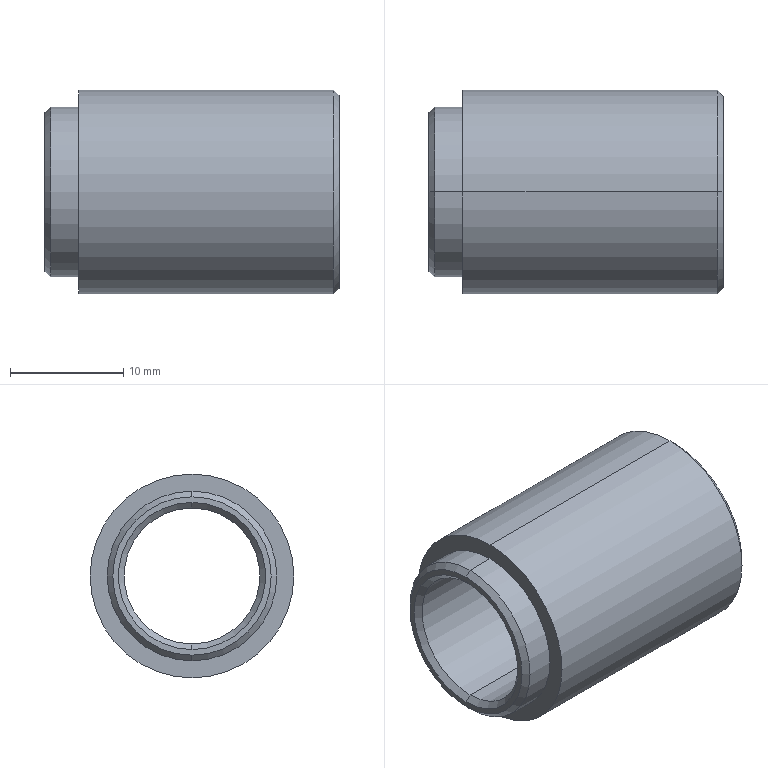Part | STEP file | 8XS210010 | 1 solid | 17 faces | box 26 x 18 x 18 mm | volume 3420 mm3 | cone 8 | cylinder 6 | plane 3 | commonest cylinder face diameters 12 x2 15 x2 18 x2
STEP:
#1=CARTESIAN_POINT('',(0.,0.,0.));
#2=DIRECTION('',(0.,0.,1.));
#3=DIRECTION('',(1.,0.,0.));
#4=AXIS2_PLACEMENT_3D('',#1,#2,#3);
#5=CARTESIAN_POINT('',(3.,0.,-9.));
#6=VERTEX_POINT('',#5);
#7=CARTESIAN_POINT('',(3.,0.,9.));
#8=VERTEX_POINT('',#7);
#9=CARTESIAN_POINT('',(3.,0.,0.));
#10=DIRECTION('',(1.,0.,0.));
#11=DIRECTION('',(0.,0.,-1.));
#12=AXIS2_PLACEMENT_3D('',#9,#10,#11);
#13=CIRCLE('',#12,9.);
#14=CARTESIAN_POINT('',(14.5,0.,0.));
#15=DIRECTION('',(1.,0.,0.));
#16=DIRECTION('',(0.,0.,-1.));
#17=AXIS2_PLACEMENT_3D('',#14,#15,#16);
#18=CYLINDRICAL_SURFACE('',#17,9.);
#19=CARTESIAN_POINT('',(0.,-11.5));
#20=DIRECTION('',(1.,0.));
#21=VECTOR('',#20,1.);
#22=LINE('',#19,#21);
#23=(GEOMETRIC_REPRESENTATION_CONTEXT(2)PARAMETRIC_REPRESENTATION_CONTEXT()REPRESENTATION_CONTEXT('',''));
#24=DEFINITIONAL_REPRESENTATION('',(#22),#23);
#25=PCURVE('',#18,#24);
#26=CARTESIAN_POINT('',(3.,8.25,0.));
#27=DIRECTION('',(-1.,0.,0.));
#28=DIRECTION('',(0.,0.,1.));
#29=AXIS2_PLACEMENT_3D('',#26,#27,#28);
#30=PLANE('',#29);
#31=CARTESIAN_POINT('',(-9.,-8.25));
#32=CARTESIAN_POINT('',(-9.,7.338));
#33=CARTESIAN_POINT('',(4.5,-0.4558));
#34=CARTESIAN_POINT('',(18.,-8.25));
#35=CARTESIAN_POINT('',(4.5,-16.044));
#36=CARTESIAN_POINT('',(-9.,-23.838));
#37=CARTESIAN_POINT('',(-9.,-8.25));
#38=(BOUNDED_CURVE()B_SPLINE_CURVE(2,(#31,#32,#33,#34,#35,#36,#37),.UNSPECIFIED.,.T.,.F.)B_SPLINE_CURVE_WITH_KNOTS((1,2,2,2,2,1),(-2.094,0.,2.094,4.189,6.283,8.378),.UNSPECIFIED.)CURVE()GEOMETRIC_REPRESENTATION_ITEM()RATIONAL_B_SPLINE_CURVE((1.,0.5,1.,0.5,1.,0.5,1.))REPRESENTATION_ITEM(''));
#39=(GEOMETRIC_REPRESENTATION_CONTEXT(2)PARAMETRIC_REPRESENTATION_CONTEXT()REPRESENTATION_CONTEXT('',''));
#40=DEFINITIONAL_REPRESENTATION('',(#38),#39);
#41=PCURVE('',#30,#40);
#42=SURFACE_CURVE('',#13,(#25,#41),.PCURVE_S1.);
#43=EDGE_CURVE('',#6,#8,#42,.T.);
#44=ORIENTED_EDGE('',*,*,#43,.T.);
#45=CARTESIAN_POINT('',(25.5,0.,9.));
#46=VERTEX_POINT('',#45);
#47=CARTESIAN_POINT('',(14.5,0.,9.));
#48=DIRECTION('',(1.,0.,0.));
#49=VECTOR('',#48,1.);
#50=LINE('',#47,#49);
#51=CARTESIAN_POINT('',(3.142,0.));
#52=DIRECTION('',(0.,1.));
#53=VECTOR('',#52,1.);
#54=LINE('',#51,#53);
#55=(GEOMETRIC_REPRESENTATION_CONTEXT(2)PARAMETRIC_REPRESENTATION_CONTEXT()REPRESENTATION_CONTEXT('',''));
#56=DEFINITIONAL_REPRESENTATION('',(#54),#55);
#57=PCURVE('',#18,#56);
#58=CARTESIAN_POINT('',(14.5,0.,0.));
#59=DIRECTION('',(1.,0.,0.));
#60=DIRECTION('',(0.,0.,-1.));
#61=AXIS2_PLACEMENT_3D('',#58,#59,#60);
#62=CYLINDRICAL_SURFACE('',#61,9.);
#63=CARTESIAN_POINT('',(3.142,0.));
#64=DIRECTION('',(0.,1.));
#65=VECTOR('',#64,1.);
#66=LINE('',#63,#65);
#67=(GEOMETRIC_REPRESENTATION_CONTEXT(2)PARAMETRIC_REPRESENTATION_CONTEXT()REPRESENTATION_CONTEXT('',''));
#68=DEFINITIONAL_REPRESENTATION('',(#66),#67);
#69=PCURVE('',#62,#68);
#70=SURFACE_CURVE('',#50,(#57,#69),.PCURVE_S1.);
#71=EDGE_CURVE('',#8,#46,#70,.T.);
#72=ORIENTED_EDGE('',*,*,#71,.T.);
#73=CARTESIAN_POINT('',(25.5,0.,-9.));
#74=VERTEX_POINT('',#73);
#75=CARTESIAN_POINT('',(25.5,0.,0.));
#76=DIRECTION('',(-1.,0.,0.));
#77=DIRECTION('',(0.,0.,-1.));
#78=AXIS2_PLACEMENT_3D('',#75,#76,#77);
#79=CIRCLE('',#78,9.);
#80=CARTESIAN_POINT('',(6.283,11.));
#81=DIRECTION('',(-1.,0.));
#82=VECTOR('',#81,1.);
#83=LINE('',#80,#82);
#84=(GEOMETRIC_REPRESENTATION_CONTEXT(2)PARAMETRIC_REPRESENTATION_CONTEXT()REPRESENTATION_CONTEXT('',''));
#85=DEFINITIONAL_REPRESENTATION('',(#83),#84);
#86=PCURVE('',#18,#85);
#87=CARTESIAN_POINT('',(25.5,0.,0.));
#88=DIRECTION('',(-1.,0.,0.));
#89=DIRECTION('',(0.,0.,1.));
#90=AXIS2_PLACEMENT_3D('',#87,#88,#89);
#91=CONICAL_SURFACE('',#90,9.,0.7854);
#92=CARTESIAN_POINT('',(-3.142,0.));
#93=DIRECTION('',(1.,0.));
#94=VECTOR('',#93,1.);
#95=LINE('',#92,#94);
#96=(GEOMETRIC_REPRESENTATION_CONTEXT(2)PARAMETRIC_REPRESENTATION_CONTEXT()REPRESENTATION_CONTEXT('',''));
#97=DEFINITIONAL_REPRESENTATION('',(#95),#96);
#98=PCURVE('',#91,#97);
#99=SURFACE_CURVE('',#79,(#86,#98),.PCURVE_S1.);
#100=EDGE_CURVE('',#46,#74,#99,.T.);
#101=ORIENTED_EDGE('',*,*,#100,.T.);
#102=CARTESIAN_POINT('',(14.5,0.,-9.));
#103=DIRECTION('',(1.,0.,0.));
#104=VECTOR('',#103,1.);
#105=LINE('',#102,#104);
#106=CARTESIAN_POINT('',(0.,0.));
#107=DIRECTION('',(0.,1.));
#108=VECTOR('',#107,1.);
#109=LINE('',#106,#108);
#110=(GEOMETRIC_REPRESENTATION_CONTEXT(2)PARAMETRIC_REPRESENTATION_CONTEXT()REPRESENTATION_CONTEXT('',''));
#111=DEFINITIONAL_REPRESENTATION('',(#109),#110);
#112=PCURVE('',#18,#111);
#113=CARTESIAN_POINT('',(6.283,0.));
#114=DIRECTION('',(0.,1.));
#115=VECTOR('',#114,1.);
#116=LINE('',#113,#115);
#117=(GEOMETRIC_REPRESENTATION_CONTEXT(2)PARAMETRIC_REPRESENTATION_CONTEXT()REPRESENTATION_CONTEXT('',''));
#118=DEFINITIONAL_REPRESENTATION('',(#116),#117);
#119=PCURVE('',#62,#118);
#120=SURFACE_CURVE('',#105,(#112,#119),.PCURVE_S1.);
#121=EDGE_CURVE('',#6,#74,#120,.T.);
#122=ORIENTED_EDGE('',*,*,#121,.F.);
#123=EDGE_LOOP('',(#44,#72,#101,#122));
#124=FACE_BOUND('',#123,.T.);
#125=ADVANCED_FACE('',(#124),#18,.T.);
#126=CARTESIAN_POINT('',(26.,0.,8.5));
#127=VERTEX_POINT('',#126);
#128=CARTESIAN_POINT('',(26.,0.,-8.5));
#129=VERTEX_POINT('',#128);
#130=CARTESIAN_POINT('',(26.,0.,0.));
#131=DIRECTION('',(-1.,0.,0.));
#132=DIRECTION('',(0.,0.,1.));
#133=AXIS2_PLACEMENT_3D('',#130,#131,#132);
#134=CIRCLE('',#133,8.5);
#135=CARTESIAN_POINT('',(0.,-0.5));
#136=DIRECTION('',(1.,0.));
#137=VECTOR('',#136,1.);
#138=LINE('',#135,#137);
#139=(GEOMETRIC_REPRESENTATION_CONTEXT(2)PARAMETRIC_REPRESENTATION_CONTEXT()REPRESENTATION_CONTEXT('',''));
#140=DEFINITIONAL_REPRESENTATION('',(#138),#139);
#141=PCURVE('',#91,#140);
#142=CARTESIAN_POINT('',(26.,7.5,0.));
#143=DIRECTION('',(1.,0.,0.));
#144=DIRECTION('',(0.,0.,-1.));
#145=AXIS2_PLACEMENT_3D('',#142,#143,#144);
#146=PLANE('',#145);
#147=CARTESIAN_POINT('',(-8.5,-7.5));
#148=CARTESIAN_POINT('',(-8.5,7.222));
#149=CARTESIAN_POINT('',(4.25,-0.1388));
#150=CARTESIAN_POINT('',(17.,-7.5));
#151=CARTESIAN_POINT('',(4.25,-14.861));
#152=CARTESIAN_POINT('',(-8.5,-22.222));
#153=CARTESIAN_POINT('',(-8.5,-7.5));
#154=(BOUNDED_CURVE()B_SPLINE_CURVE(2,(#147,#148,#149,#150,#151,#152,#153),.UNSPECIFIED.,.T.,.F.)B_SPLINE_CURVE_WITH_KNOTS((1,2,2,2,2,1),(-2.094,0.,2.094,4.189,6.283,8.378),.UNSPECIFIED.)CURVE()GEOMETRIC_REPRESENTATION_ITEM()RATIONAL_B_SPLINE_CURVE((1.,0.5,1.,0.5,1.,0.5,1.))REPRESENTATION_ITEM(''));
#155=(GEOMETRIC_REPRESENTATION_CONTEXT(2)PARAMETRIC_REPRESENTATION_CONTEXT()REPRESENTATION_CONTEXT('',''));
#156=DEFINITIONAL_REPRESENTATION('',(#154),#155);
#157=PCURVE('',#146,#156);
#158=SURFACE_CURVE('',#134,(#141,#157),.PCURVE_S1.);
#159=EDGE_CURVE('',#127,#129,#158,.T.);
#160=ORIENTED_EDGE('',*,*,#159,.T.);
#161=CARTESIAN_POINT('',(25.5,0.,-9.));
#162=DIRECTION('',(-0.7071,0.,-0.7071));
#163=VECTOR('',#162,1.);
#164=LINE('',#161,#163);
#165=CARTESIAN_POINT('',(3.142,0.));
#166=DIRECTION('',(0.,1.));
#167=VECTOR('',#166,1.);
#168=LINE('',#165,#167);
#169=(GEOMETRIC_REPRESENTATION_CONTEXT(2)PARAMETRIC_REPRESENTATION_CONTEXT()REPRESENTATION_CONTEXT('',''));
#170=DEFINITIONAL_REPRESENTATION('',(#168),#169);
#171=PCURVE('',#91,#170);
#172=CARTESIAN_POINT('',(25.5,0.,0.));
#173=DIRECTION('',(-1.,0.,0.));
#174=DIRECTION('',(0.,0.,1.));
#175=AXIS2_PLACEMENT_3D('',#172,#173,#174);
#176=CONICAL_SURFACE('',#175,9.,0.7854);
#177=CARTESIAN_POINT('',(3.142,0.));
#178=DIRECTION('',(0.,1.));
#179=VECTOR('',#178,1.);
#180=LINE('',#177,#179);
#181=(GEOMETRIC_REPRESENTATION_CONTEXT(2)PARAMETRIC_REPRESENTATION_CONTEXT()REPRESENTATION_CONTEXT('',''));
#182=DEFINITIONAL_REPRESENTATION('',(#180),#181);
#183=PCURVE('',#176,#182);
#184=SURFACE_CURVE('',#164,(#171,#183),.PCURVE_S1.);
#185=EDGE_CURVE('',#129,#74,#184,.T.);
#186=ORIENTED_EDGE('',*,*,#185,.T.);
#187=ORIENTED_EDGE('',*,*,#100,.F.);
#188=CARTESIAN_POINT('',(25.5,0.,9.));
#189=DIRECTION('',(-0.7071,0.,0.7071));
#190=VECTOR('',#189,1.);
#191=LINE('',#188,#190);
#192=CARTESIAN_POINT('',(0.,0.));
#193=DIRECTION('',(0.,1.));
#194=VECTOR('',#193,1.);
#195=LINE('',#192,#194);
#196=(GEOMETRIC_REPRESENTATION_CONTEXT(2)PARAMETRIC_REPRESENTATION_CONTEXT()REPRESENTATION_CONTEXT('',''));
#197=DEFINITIONAL_REPRESENTATION('',(#195),#196);
#198=PCURVE('',#91,#197);
#199=CARTESIAN_POINT('',(6.283,0.));
#200=DIRECTION('',(0.,1.));
#201=VECTOR('',#200,1.);
#202=LINE('',#199,#201);
#203=(GEOMETRIC_REPRESENTATION_CONTEXT(2)PARAMETRIC_REPRESENTATION_CONTEXT()REPRESENTATION_CONTEXT('',''));
#204=DEFINITIONAL_REPRESENTATION('',(#202),#203);
#205=PCURVE('',#176,#204);
#206=SURFACE_CURVE('',#191,(#198,#205),.PCURVE_S1.);
#207=EDGE_CURVE('',#127,#46,#206,.T.);
#208=ORIENTED_EDGE('',*,*,#207,.F.);
#209=EDGE_LOOP('',(#160,#186,#187,#208));
#210=FACE_BOUND('',#209,.T.);
#211=ADVANCED_FACE('',(#210),#91,.T.);
#212=CARTESIAN_POINT('',(0.5,0.,-7.5));
#213=VERTEX_POINT('',#212);
#214=CARTESIAN_POINT('',(0.5,0.,7.5));
#215=VERTEX_POINT('',#214);
#216=CARTESIAN_POINT('',(0.5,0.,0.));
#217=DIRECTION('',(1.,0.,0.));
#218=DIRECTION('',(0.,0.,-1.));
#219=AXIS2_PLACEMENT_3D('',#216,#217,#218);
#220=CIRCLE('',#219,7.5);
#221=CARTESIAN_POINT('',(1.5,0.,0.));
#222=DIRECTION('',(1.,0.,0.));
#223=DIRECTION('',(0.,0.,-1.));
#224=AXIS2_PLACEMENT_3D('',#221,#222,#223);
#225=CYLINDRICAL_SURFACE('',#224,7.5);
#226=CARTESIAN_POINT('',(0.,-1.));
#227=DIRECTION('',(1.,0.));
#228=VECTOR('',#227,1.);
#229=LINE('',#226,#228);
#230=(GEOMETRIC_REPRESENTATION_CONTEXT(2)PARAMETRIC_REPRESENTATION_CONTEXT()REPRESENTATION_CONTEXT('',''));
#231=DEFINITIONAL_REPRESENTATION('',(#229),#230);
#232=PCURVE('',#225,#231);
#233=CARTESIAN_POINT('',(0.5,0.,0.));
#234=DIRECTION('',(1.,0.,0.));
#235=DIRECTION('',(0.,0.,-1.));
#236=AXIS2_PLACEMENT_3D('',#233,#234,#235);
#237=CONICAL_SURFACE('',#236,7.5,0.7854);
#238=CARTESIAN_POINT('',(0.,0.));
#239=DIRECTION('',(1.,0.));
#240=VECTOR('',#239,1.);
#241=LINE('',#238,#240);
#242=(GEOMETRIC_REPRESENTATION_CONTEXT(2)PARAMETRIC_REPRESENTATION_CONTEXT()REPRESENTATION_CONTEXT('',''));
#243=DEFINITIONAL_REPRESENTATION('',(#241),#242);
#244=PCURVE('',#237,#243);
#245=SURFACE_CURVE('',#220,(#232,#244),.PCURVE_S1.);
#246=EDGE_CURVE('',#213,#215,#245,.T.);
#247=ORIENTED_EDGE('',*,*,#246,.T.);
#248=CARTESIAN_POINT('',(3.,0.,7.5));
#249=VERTEX_POINT('',#248);
#250=CARTESIAN_POINT('',(1.5,0.,7.5));
#251=DIRECTION('',(1.,0.,0.));
#252=VECTOR('',#251,1.);
#253=LINE('',#250,#252);
#254=CARTESIAN_POINT('',(3.142,0.));
#255=DIRECTION('',(0.,1.));
#256=VECTOR('',#255,1.);
#257=LINE('',#254,#256);
#258=(GEOMETRIC_REPRESENTATION_CONTEXT(2)PARAMETRIC_REPRESENTATION_CONTEXT()REPRESENTATION_CONTEXT('',''));
#259=DEFINITIONAL_REPRESENTATION('',(#257),#258);
#260=PCURVE('',#225,#259);
#261=CARTESIAN_POINT('',(1.5,0.,0.));
#262=DIRECTION('',(1.,0.,0.));
#263=DIRECTION('',(0.,0.,-1.));
#264=AXIS2_PLACEMENT_3D('',#261,#262,#263);
#265=CYLINDRICAL_SURFACE('',#264,7.5);
#266=CARTESIAN_POINT('',(3.142,0.));
#267=DIRECTION('',(0.,1.));
#268=VECTOR('',#267,1.);
#269=LINE('',#266,#268);
#270=(GEOMETRIC_REPRESENTATION_CONTEXT(2)PARAMETRIC_REPRESENTATION_CONTEXT()REPRESENTATION_CONTEXT('',''));
#271=DEFINITIONAL_REPRESENTATION('',(#269),#270);
#272=PCURVE('',#265,#271);
#273=SURFACE_CURVE('',#253,(#260,#272),.PCURVE_S1.);
#274=EDGE_CURVE('',#215,#249,#273,.T.);
#275=ORIENTED_EDGE('',*,*,#274,.T.);
#276=CARTESIAN_POINT('',(3.,0.,-7.5));
#277=VERTEX_POINT('',#276);
#278=CARTESIAN_POINT('',(3.,0.,0.));
#279=DIRECTION('',(1.,0.,0.));
#280=DIRECTION('',(0.,0.,-1.));
#281=AXIS2_PLACEMENT_3D('',#278,#279,#280);
#282=CIRCLE('',#281,7.5);
#283=CARTESIAN_POINT('',(0.,1.5));
#284=DIRECTION('',(1.,0.));
#285=VECTOR('',#284,1.);
#286=LINE('',#283,#285);
#287=(GEOMETRIC_REPRESENTATION_CONTEXT(2)PARAMETRIC_REPRESENTATION_CONTEXT()REPRESENTATION_CONTEXT('',''));
#288=DEFINITIONAL_REPRESENTATION('',(#286),#287);
#289=PCURVE('',#225,#288);
#290=CARTESIAN_POINT('',(-7.5,-8.25));
#291=CARTESIAN_POINT('',(-7.5,4.74));
#292=CARTESIAN_POINT('',(3.75,-1.755));
#293=CARTESIAN_POINT('',(15.,-8.25));
#294=CARTESIAN_POINT('',(3.75,-14.745));
#295=CARTESIAN_POINT('',(-7.5,-21.24));
#296=CARTESIAN_POINT('',(-7.5,-8.25));
#297=(BOUNDED_CURVE()B_SPLINE_CURVE(2,(#290,#291,#292,#293,#294,#295,#296),.UNSPECIFIED.,.T.,.F.)B_SPLINE_CURVE_WITH_KNOTS((1,2,2,2,2,1),(-2.094,0.,2.094,4.189,6.283,8.378),.UNSPECIFIED.)CURVE()GEOMETRIC_REPRESENTATION_ITEM()RATIONAL_B_SPLINE_CURVE((1.,0.5,1.,0.5,1.,0.5,1.))REPRESENTATION_ITEM(''));
#298=(GEOMETRIC_REPRESENTATION_CONTEXT(2)PARAMETRIC_REPRESENTATION_CONTEXT()REPRESENTATION_CONTEXT('',''));
#299=DEFINITIONAL_REPRESENTATION('',(#297),#298);
#300=PCURVE('',#30,#299);
#301=SURFACE_CURVE('',#282,(#289,#300),.PCURVE_S1.);
#302=EDGE_CURVE('',#277,#249,#301,.T.);
#303=ORIENTED_EDGE('',*,*,#302,.F.);
#304=CARTESIAN_POINT('',(1.5,0.,-7.5));
#305=DIRECTION('',(1.,0.,0.));
#306=VECTOR('',#305,1.);
#307=LINE('',#304,#306);
#308=CARTESIAN_POINT('',(0.,0.));
#309=DIRECTION('',(0.,1.));
#310=VECTOR('',#309,1.);
#311=LINE('',#308,#310);
#312=(GEOMETRIC_REPRESENTATION_CONTEXT(2)PARAMETRIC_REPRESENTATION_CONTEXT()REPRESENTATION_CONTEXT('',''));
#313=DEFINITIONAL_REPRESENTATION('',(#311),#312);
#314=PCURVE('',#225,#313);
#315=CARTESIAN_POINT('',(6.283,0.));
#316=DIRECTION('',(0.,1.));
#317=VECTOR('',#316,1.);
#318=LINE('',#315,#317);
#319=(GEOMETRIC_REPRESENTATION_CONTEXT(2)PARAMETRIC_REPRESENTATION_CONTEXT()REPRESENTATION_CONTEXT('',''));
#320=DEFINITIONAL_REPRESENTATION('',(#318),#319);
#321=PCURVE('',#265,#320);
#322=SURFACE_CURVE('',#307,(#314,#321),.PCURVE_S1.);
#323=EDGE_CURVE('',#213,#277,#322,.T.);
#324=ORIENTED_EDGE('',*,*,#323,.F.);
#325=EDGE_LOOP('',(#247,#275,#303,#324));
#326=FACE_BOUND('',#325,.T.);
#327=ADVANCED_FACE('',(#326),#225,.T.);
#328=CARTESIAN_POINT('',(25.5,0.,-6.));
#329=VERTEX_POINT('',#328);
#330=CARTESIAN_POINT('',(26.,0.,-6.5));
#331=VERTEX_POINT('',#330);
#332=CARTESIAN_POINT('',(26.,0.,-6.5));
#333=DIRECTION('',(0.7071,0.,-0.7071));
#334=VECTOR('',#333,1.);
#335=LINE('',#332,#334);
#336=CARTESIAN_POINT('',(26.,0.,0.));
#337=DIRECTION('',(1.,0.,0.));
#338=DIRECTION('',(0.,0.,-1.));
#339=AXIS2_PLACEMENT_3D('',#336,#337,#338);
#340=CONICAL_SURFACE('',#339,6.5,0.7854);
#341=CARTESIAN_POINT('',(6.283,0.));
#342=DIRECTION('',(0.,1.));
#343=VECTOR('',#342,1.);
#344=LINE('',#341,#343);
#345=(GEOMETRIC_REPRESENTATION_CONTEXT(2)PARAMETRIC_REPRESENTATION_CONTEXT()REPRESENTATION_CONTEXT('',''));
#346=DEFINITIONAL_REPRESENTATION('',(#344),#345);
#347=PCURVE('',#340,#346);
#348=CARTESIAN_POINT('',(26.,0.,0.));
#349=DIRECTION('',(1.,0.,0.));
#350=DIRECTION('',(0.,0.,-1.));
#351=AXIS2_PLACEMENT_3D('',#348,#349,#350);
#352=CONICAL_SURFACE('',#351,6.5,0.7854);
#353=CARTESIAN_POINT('',(0.,0.));
#354=DIRECTION('',(0.,1.));
#355=VECTOR('',#354,1.);
#356=LINE('',#353,#355);
#357=(GEOMETRIC_REPRESENTATION_CONTEXT(2)PARAMETRIC_REPRESENTATION_CONTEXT()REPRESENTATION_CONTEXT('',''));
#358=DEFINITIONAL_REPRESENTATION('',(#356),#357);
#359=PCURVE('',#352,#358);
#360=SURFACE_CURVE('',#335,(#347,#359),.PCURVE_S1.);
#361=EDGE_CURVE('',#329,#331,#360,.T.);
#362=ORIENTED_EDGE('',*,*,#361,.T.);
#363=CARTESIAN_POINT('',(26.,0.,6.5));
#364=VERTEX_POINT('',#363);
#365=CARTESIAN_POINT('',(26.,0.,0.));
#366=DIRECTION('',(-1.,0.,0.));
#367=DIRECTION('',(0.,0.,-1.));
#368=AXIS2_PLACEMENT_3D('',#365,#366,#367);
#369=CIRCLE('',#368,6.5);
#370=CARTESIAN_POINT('',(6.283,0.));
#371=DIRECTION('',(-1.,0.));
#372=VECTOR('',#371,1.);
#373=LINE('',#370,#372);
#374=(GEOMETRIC_REPRESENTATION_CONTEXT(2)PARAMETRIC_REPRESENTATION_CONTEXT()REPRESENTATION_CONTEXT('',''));
#375=DEFINITIONAL_REPRESENTATION('',(#373),#374);
#376=PCURVE('',#340,#375);
#377=CARTESIAN_POINT('',(6.5,-7.5));
#378=CARTESIAN_POINT('',(6.5,-18.758));
#379=CARTESIAN_POINT('',(-3.25,-13.129));
#380=CARTESIAN_POINT('',(-13.,-7.5));
#381=CARTESIAN_POINT('',(-3.25,-1.871));
#382=CARTESIAN_POINT('',(6.5,3.758));
#383=CARTESIAN_POINT('',(6.5,-7.5));
#384=(BOUNDED_CURVE()B_SPLINE_CURVE(2,(#377,#378,#379,#380,#381,#382,#383),.UNSPECIFIED.,.T.,.F.)B_SPLINE_CURVE_WITH_KNOTS((1,2,2,2,2,1),(-2.094,0.,2.094,4.189,6.283,8.378),.UNSPECIFIED.)CURVE()GEOMETRIC_REPRESENTATION_ITEM()RATIONAL_B_SPLINE_CURVE((1.,0.5,1.,0.5,1.,0.5,1.))REPRESENTATION_ITEM(''));
#385=(GEOMETRIC_REPRESENTATION_CONTEXT(2)PARAMETRIC_REPRESENTATION_CONTEXT()REPRESENTATION_CONTEXT('',''));
#386=DEFINITIONAL_REPRESENTATION('',(#384),#385);
#387=PCURVE('',#146,#386);
#388=SURFACE_CURVE('',#369,(#376,#387),.PCURVE_S1.);
#389=EDGE_CURVE('',#331,#364,#388,.T.);
#390=ORIENTED_EDGE('',*,*,#389,.T.);
#391=CARTESIAN_POINT('',(25.5,0.,6.));
#392=VERTEX_POINT('',#391);
#393=CARTESIAN_POINT('',(26.,0.,6.5));
#394=DIRECTION('',(0.7071,0.,0.7071));
#395=VECTOR('',#394,1.);
#396=LINE('',#393,#395);
#397=CARTESIAN_POINT('',(3.142,0.));
#398=DIRECTION('',(0.,1.));
#399=VECTOR('',#398,1.);
#400=LINE('',#397,#399);
#401=(GEOMETRIC_REPRESENTATION_CONTEXT(2)PARAMETRIC_REPRESENTATION_CONTEXT()REPRESENTATION_CONTEXT('',''));
#402=DEFINITIONAL_REPRESENTATION('',(#400),#401);
#403=PCURVE('',#340,#402);
#404=CARTESIAN_POINT('',(3.142,0.));
#405=DIRECTION('',(0.,1.));
#406=VECTOR('',#405,1.);
#407=LINE('',#404,#406);
#408=(GEOMETRIC_REPRESENTATION_CONTEXT(2)PARAMETRIC_REPRESENTATION_CONTEXT()REPRESENTATION_CONTEXT('',''));
#409=DEFINITIONAL_REPRESENTATION('',(#407),#408);
#410=PCURVE('',#352,#409);
#411=SURFACE_CURVE('',#396,(#403,#410),.PCURVE_S1.);
#412=EDGE_CURVE('',#392,#364,#411,.T.);
#413=ORIENTED_EDGE('',*,*,#412,.F.);
#414=CARTESIAN_POINT('',(25.5,0.,0.));
#415=DIRECTION('',(1.,0.,0.));
#416=DIRECTION('',(0.,-1.,0.));
#417=AXIS2_PLACEMENT_3D('',#414,#415,#416);
#418=CIRCLE('',#417,6.);
#419=CARTESIAN_POINT('',(-1.571,-0.5));
#420=DIRECTION('',(1.,0.));
#421=VECTOR('',#420,1.);
#422=LINE('',#419,#421);
#423=(GEOMETRIC_REPRESENTATION_CONTEXT(2)PARAMETRIC_REPRESENTATION_CONTEXT()REPRESENTATION_CONTEXT('',''));
#424=DEFINITIONAL_REPRESENTATION('',(#422),#423);
#425=PCURVE('',#340,#424);
#426=CARTESIAN_POINT('',(13.,0.,0.));
#427=DIRECTION('',(1.,0.,0.));
#428=DIRECTION('',(0.,0.,-1.));
#429=AXIS2_PLACEMENT_3D('',#426,#427,#428);
#430=CYLINDRICAL_SURFACE('',#429,6.);
#431=CARTESIAN_POINT('',(-1.571,12.5));
#432=DIRECTION('',(1.,0.));
#433=VECTOR('',#432,1.);
#434=LINE('',#431,#433);
#435=(GEOMETRIC_REPRESENTATION_CONTEXT(2)PARAMETRIC_REPRESENTATION_CONTEXT()REPRESENTATION_CONTEXT('',''));
#436=DEFINITIONAL_REPRESENTATION('',(#434),#435);
#437=PCURVE('',#430,#436);
#438=SURFACE_CURVE('',#418,(#425,#437),.PCURVE_S1.);
#439=EDGE_CURVE('',#392,#329,#438,.T.);
#440=ORIENTED_EDGE('',*,*,#439,.T.);
#441=EDGE_LOOP('',(#362,#390,#413,#440));
#442=FACE_BOUND('',#441,.F.);
#443=ADVANCED_FACE('',(#442),#340,.F.);
#444=CARTESIAN_POINT('',(0.,0.,-7.));
#445=VERTEX_POINT('',#444);
#446=CARTESIAN_POINT('',(0.,0.,7.));
#447=VERTEX_POINT('',#446);
#448=CARTESIAN_POINT('',(0.,0.,0.));
#449=DIRECTION('',(1.,0.,0.));
#450=DIRECTION('',(0.,0.,-1.));
#451=AXIS2_PLACEMENT_3D('',#448,#449,#450);
#452=CIRCLE('',#451,7.);
#453=CARTESIAN_POINT('',(0.,-0.5));
#454=DIRECTION('',(1.,0.));
#455=VECTOR('',#454,1.);
#456=LINE('',#453,#455);
#457=(GEOMETRIC_REPRESENTATION_CONTEXT(2)PARAMETRIC_REPRESENTATION_CONTEXT()REPRESENTATION_CONTEXT('',''));
#458=DEFINITIONAL_REPRESENTATION('',(#456),#457);
#459=PCURVE('',#237,#458);
#460=CARTESIAN_POINT('',(0.,6.75,0.));
#461=DIRECTION('',(-1.,0.,0.));
#462=DIRECTION('',(0.,0.,1.));
#463=AXIS2_PLACEMENT_3D('',#460,#461,#462);
#464=PLANE('',#463);
#465=CARTESIAN_POINT('',(-7.,-6.75));
#466=CARTESIAN_POINT('',(-7.,5.374));
#467=CARTESIAN_POINT('',(3.5,-0.6878));
#468=CARTESIAN_POINT('',(14.,-6.75));
#469=CARTESIAN_POINT('',(3.5,-12.812));
#470=CARTESIAN_POINT('',(-7.,-18.874));
#471=CARTESIAN_POINT('',(-7.,-6.75));
#472=(BOUNDED_CURVE()B_SPLINE_CURVE(2,(#465,#466,#467,#468,#469,#470,#471),.UNSPECIFIED.,.T.,.F.)B_SPLINE_CURVE_WITH_KNOTS((1,2,2,2,2,1),(-2.094,0.,2.094,4.189,6.283,8.378),.UNSPECIFIED.)CURVE()GEOMETRIC_REPRESENTATION_ITEM()RATIONAL_B_SPLINE_CURVE((1.,0.5,1.,0.5,1.,0.5,1.))REPRESENTATION_ITEM(''));
#473=(GEOMETRIC_REPRESENTATION_CONTEXT(2)PARAMETRIC_REPRESENTATION_CONTEXT()REPRESENTATION_CONTEXT('',''));
#474=DEFINITIONAL_REPRESENTATION('',(#472),#473);
#475=PCURVE('',#464,#474);
#476=SURFACE_CURVE('',#452,(#459,#475),.PCURVE_S1.);
#477=EDGE_CURVE('',#445,#447,#476,.T.);
#478=ORIENTED_EDGE('',*,*,#477,.T.);
#479=CARTESIAN_POINT('',(0.5,0.,7.5));
#480=DIRECTION('',(0.7071,0.,0.7071));
#481=VECTOR('',#480,1.);
#482=LINE('',#479,#481);
#483=CARTESIAN_POINT('',(3.142,0.));
#484=DIRECTION('',(0.,1.));
#485=VECTOR('',#484,1.);
#486=LINE('',#483,#485);
#487=(GEOMETRIC_REPRESENTATION_CONTEXT(2)PARAMETRIC_REPRESENTATION_CONTEXT()REPRESENTATION_CONTEXT('',''));
#488=DEFINITIONAL_REPRESENTATION('',(#486),#487);
#489=PCURVE('',#237,#488);
#490=CARTESIAN_POINT('',(0.5,0.,0.));
#491=DIRECTION('',(1.,0.,0.));
#492=DIRECTION('',(0.,0.,-1.));
#493=AXIS2_PLACEMENT_3D('',#490,#491,#492);
#494=CONICAL_SURFACE('',#493,7.5,0.7854);
#495=CARTESIAN_POINT('',(3.142,0.));
#496=DIRECTION('',(0.,1.));
#497=VECTOR('',#496,1.);
#498=LINE('',#495,#497);
#499=(GEOMETRIC_REPRESENTATION_CONTEXT(2)PARAMETRIC_REPRESENTATION_CONTEXT()REPRESENTATION_CONTEXT('',''));
#500=DEFINITIONAL_REPRESENTATION('',(#498),#499);
#501=PCURVE('',#494,#500);
#502=SURFACE_CURVE('',#482,(#489,#501),.PCURVE_S1.);
#503=EDGE_CURVE('',#447,#215,#502,.T.);
#504=ORIENTED_EDGE('',*,*,#503,.T.);
#505=ORIENTED_EDGE('',*,*,#246,.F.);
#506=CARTESIAN_POINT('',(0.5,0.,-7.5));
#507=DIRECTION('',(0.7071,0.,-0.7071));
#508=VECTOR('',#507,1.);
#509=LINE('',#506,#508);
#510=CARTESIAN_POINT('',(0.,0.));
#511=DIRECTION('',(0.,1.));
#512=VECTOR('',#511,1.);
#513=LINE('',#510,#512);
#514=(GEOMETRIC_REPRESENTATION_CONTEXT(2)PARAMETRIC_REPRESENTATION_CONTEXT()REPRESENTATION_CONTEXT('',''));
#515=DEFINITIONAL_REPRESENTATION('',(#513),#514);
#516=PCURVE('',#237,#515);
#517=CARTESIAN_POINT('',(6.283,0.));
#518=DIRECTION('',(0.,1.));
#519=VECTOR('',#518,1.);
#520=LINE('',#517,#519);
#521=(GEOMETRIC_REPRESENTATION_CONTEXT(2)PARAMETRIC_REPRESENTATION_CONTEXT()REPRESENTATION_CONTEXT('',''));
#522=DEFINITIONAL_REPRESENTATION('',(#520),#521);
#523=PCURVE('',#494,#522);
#524=SURFACE_CURVE('',#509,(#516,#523),.PCURVE_S1.);
#525=EDGE_CURVE('',#445,#213,#524,.T.);
#526=ORIENTED_EDGE('',*,*,#525,.F.);
#527=EDGE_LOOP('',(#478,#504,#505,#526));
#528=FACE_BOUND('',#527,.T.);
#529=ADVANCED_FACE('',(#528),#237,.T.);
#530=CARTESIAN_POINT('',(0.5,0.,-6.));
#531=VERTEX_POINT('',#530);
#532=CARTESIAN_POINT('',(13.,0.,-6.));
#533=DIRECTION('',(1.,0.,0.));
#534=VECTOR('',#533,1.);
#535=LINE('',#532,#534);
#536=CARTESIAN_POINT('',(6.283,0.));
#537=DIRECTION('',(0.,1.));
#538=VECTOR('',#537,1.);
#539=LINE('',#536,#538);
#540=(GEOMETRIC_REPRESENTATION_CONTEXT(2)PARAMETRIC_REPRESENTATION_CONTEXT()REPRESENTATION_CONTEXT('',''));
#541=DEFINITIONAL_REPRESENTATION('',(#539),#540);
#542=PCURVE('',#430,#541);
#543=CARTESIAN_POINT('',(13.,0.,0.));
#544=DIRECTION('',(1.,0.,0.));
#545=DIRECTION('',(0.,0.,-1.));
#546=AXIS2_PLACEMENT_3D('',#543,#544,#545);
#547=CYLINDRICAL_SURFACE('',#546,6.);
#548=CARTESIAN_POINT('',(0.,0.));
#549=DIRECTION('',(0.,1.));
#550=VECTOR('',#549,1.);
#551=LINE('',#548,#550);
#552=(GEOMETRIC_REPRESENTATION_CONTEXT(2)PARAMETRIC_REPRESENTATION_CONTEXT()REPRESENTATION_CONTEXT('',''));
#553=DEFINITIONAL_REPRESENTATION('',(#551),#552);
#554=PCURVE('',#547,#553);
#555=SURFACE_CURVE('',#535,(#542,#554),.PCURVE_S1.);
#556=EDGE_CURVE('',#531,#329,#555,.T.);
#557=ORIENTED_EDGE('',*,*,#556,.T.);
#558=ORIENTED_EDGE('',*,*,#439,.F.);
#559=CARTESIAN_POINT('',(0.5,0.,6.));
#560=VERTEX_POINT('',#559);
#561=CARTESIAN_POINT('',(13.,0.,6.));
#562=DIRECTION('',(1.,0.,0.));
#563=VECTOR('',#562,1.);
#564=LINE('',#561,#563);
#565=CARTESIAN_POINT('',(3.142,0.));
#566=DIRECTION('',(0.,1.));
#567=VECTOR('',#566,1.);
#568=LINE('',#565,#567);
#569=(GEOMETRIC_REPRESENTATION_CONTEXT(2)PARAMETRIC_REPRESENTATION_CONTEXT()REPRESENTATION_CONTEXT('',''));
#570=DEFINITIONAL_REPRESENTATION('',(#568),#569);
#571=PCURVE('',#430,#570);
#572=CARTESIAN_POINT('',(3.142,0.));
#573=DIRECTION('',(0.,1.));
#574=VECTOR('',#573,1.);
#575=LINE('',#572,#574);
#576=(GEOMETRIC_REPRESENTATION_CONTEXT(2)PARAMETRIC_REPRESENTATION_CONTEXT()REPRESENTATION_CONTEXT('',''));
#577=DEFINITIONAL_REPRESENTATION('',(#575),#576);
#578=PCURVE('',#547,#577);
#579=SURFACE_CURVE('',#564,(#571,#578),.PCURVE_S1.);
#580=EDGE_CURVE('',#560,#392,#579,.T.);
#581=ORIENTED_EDGE('',*,*,#580,.F.);
#582=CARTESIAN_POINT('',(0.5,0.,0.));
#583=DIRECTION('',(1.,0.,0.));
#584=DIRECTION('',(0.,0.,-1.));
#585=AXIS2_PLACEMENT_3D('',#582,#583,#584);
#586=CIRCLE('',#585,6.);
#587=CARTESIAN_POINT('',(0.,-12.5));
#588=DIRECTION('',(1.,0.));
#589=VECTOR('',#588,1.);
#590=LINE('',#587,#589);
#591=(GEOMETRIC_REPRESENTATION_CONTEXT(2)PARAMETRIC_REPRESENTATION_CONTEXT()REPRESENTATION_CONTEXT('',''));
#592=DEFINITIONAL_REPRESENTATION('',(#590),#591);
#593=PCURVE('',#430,#592);
#594=CARTESIAN_POINT('',(0.,0.,0.));
#595=DIRECTION('',(-1.,0.,0.));
#596=DIRECTION('',(0.,0.,1.));
#597=AXIS2_PLACEMENT_3D('',#594,#595,#596);
#598=CONICAL_SURFACE('',#597,6.5,0.7854);
#599=CARTESIAN_POINT('',(9.425,-0.5));
#600=DIRECTION('',(-1.,0.));
#601=VECTOR('',#600,1.);
#602=LINE('',#599,#601);
#603=(GEOMETRIC_REPRESENTATION_CONTEXT(2)PARAMETRIC_REPRESENTATION_CONTEXT()REPRESENTATION_CONTEXT('',''));
#604=DEFINITIONAL_REPRESENTATION('',(#602),#603);
#605=PCURVE('',#598,#604);
#606=SURFACE_CURVE('',#586,(#593,#605),.PCURVE_S1.);
#607=EDGE_CURVE('',#560,#531,#606,.T.);
#608=ORIENTED_EDGE('',*,*,#607,.T.);
#609=EDGE_LOOP('',(#557,#558,#581,#608));
#610=FACE_BOUND('',#609,.F.);
#611=ADVANCED_FACE('',(#610),#430,.F.);
#612=CARTESIAN_POINT('',(0.,0.,6.5));
#613=VERTEX_POINT('',#612);
#614=CARTESIAN_POINT('',(0.,0.,6.5));
#615=DIRECTION('',(-0.7071,0.,0.7071));
#616=VECTOR('',#615,1.);
#617=LINE('',#614,#616);
#618=CARTESIAN_POINT('',(6.283,0.));
#619=DIRECTION('',(0.,1.));
#620=VECTOR('',#619,1.);
#621=LINE('',#618,#620);
#622=(GEOMETRIC_REPRESENTATION_CONTEXT(2)PARAMETRIC_REPRESENTATION_CONTEXT()REPRESENTATION_CONTEXT('',''));
#623=DEFINITIONAL_REPRESENTATION('',(#621),#622);
#624=PCURVE('',#598,#623);
#625=CARTESIAN_POINT('',(0.,0.,0.));
#626=DIRECTION('',(-1.,0.,0.));
#627=DIRECTION('',(0.,0.,1.));
#628=AXIS2_PLACEMENT_3D('',#625,#626,#627);
#629=CONICAL_SURFACE('',#628,6.5,0.7854);
#630=CARTESIAN_POINT('',(0.,0.));
#631=DIRECTION('',(0.,1.));
#632=VECTOR('',#631,1.);
#633=LINE('',#630,#632);
#634=(GEOMETRIC_REPRESENTATION_CONTEXT(2)PARAMETRIC_REPRESENTATION_CONTEXT()REPRESENTATION_CONTEXT('',''));
#635=DEFINITIONAL_REPRESENTATION('',(#633),#634);
#636=PCURVE('',#629,#635);
#637=SURFACE_CURVE('',#617,(#624,#636),.PCURVE_S1.);
#638=EDGE_CURVE('',#560,#613,#637,.T.);
#639=ORIENTED_EDGE('',*,*,#638,.T.);
#640=CARTESIAN_POINT('',(0.,0.,-6.5));
#641=VERTEX_POINT('',#640);
#642=CARTESIAN_POINT('',(0.,0.,0.));
#643=DIRECTION('',(1.,0.,0.));
#644=DIRECTION('',(0.,0.,1.));
#645=AXIS2_PLACEMENT_3D('',#642,#643,#644);
#646=CIRCLE('',#645,6.5);
#647=CARTESIAN_POINT('',(6.283,0.));
#648=DIRECTION('',(-1.,0.));
#649=VECTOR('',#648,1.);
#650=LINE('',#647,#649);
#651=(GEOMETRIC_REPRESENTATION_CONTEXT(2)PARAMETRIC_REPRESENTATION_CONTEXT()REPRESENTATION_CONTEXT('',''));
#652=DEFINITIONAL_REPRESENTATION('',(#650),#651);
#653=PCURVE('',#598,#652);
#654=CARTESIAN_POINT('',(6.5,-6.75));
#655=CARTESIAN_POINT('',(6.5,-18.008));
#656=CARTESIAN_POINT('',(-3.25,-12.379));
#657=CARTESIAN_POINT('',(-13.,-6.75));
#658=CARTESIAN_POINT('',(-3.25,-1.121));
#659=CARTESIAN_POINT('',(6.5,4.508));
#660=CARTESIAN_POINT('',(6.5,-6.75));
#661=(BOUNDED_CURVE()B_SPLINE_CURVE(2,(#654,#655,#656,#657,#658,#659,#660),.UNSPECIFIED.,.T.,.F.)B_SPLINE_CURVE_WITH_KNOTS((1,2,2,2,2,1),(-2.094,0.,2.094,4.189,6.283,8.378),.UNSPECIFIED.)CURVE()GEOMETRIC_REPRESENTATION_ITEM()RATIONAL_B_SPLINE_CURVE((1.,0.5,1.,0.5,1.,0.5,1.))REPRESENTATION_ITEM(''));
#662=(GEOMETRIC_REPRESENTATION_CONTEXT(2)PARAMETRIC_REPRESENTATION_CONTEXT()REPRESENTATION_CONTEXT('',''));
#663=DEFINITIONAL_REPRESENTATION('',(#661),#662);
#664=PCURVE('',#464,#663);
#665=SURFACE_CURVE('',#646,(#653,#664),.PCURVE_S1.);
#666=EDGE_CURVE('',#613,#641,#665,.T.);
#667=ORIENTED_EDGE('',*,*,#666,.T.);
#668=CARTESIAN_POINT('',(0.,0.,-6.5));
#669=DIRECTION('',(-0.7071,0.,-0.7071));
#670=VECTOR('',#669,1.);
#671=LINE('',#668,#670);
#672=CARTESIAN_POINT('',(3.142,0.));
#673=DIRECTION('',(0.,1.));
#674=VECTOR('',#673,1.);
#675=LINE('',#672,#674);
#676=(GEOMETRIC_REPRESENTATION_CONTEXT(2)PARAMETRIC_REPRESENTATION_CONTEXT()REPRESENTATION_CONTEXT('',''));
#677=DEFINITIONAL_REPRESENTATION('',(#675),#676);
#678=PCURVE('',#598,#677);
#679=CARTESIAN_POINT('',(3.142,0.));
#680=DIRECTION('',(0.,1.));
#681=VECTOR('',#680,1.);
#682=LINE('',#679,#681);
#683=(GEOMETRIC_REPRESENTATION_CONTEXT(2)PARAMETRIC_REPRESENTATION_CONTEXT()REPRESENTATION_CONTEXT('',''));
#684=DEFINITIONAL_REPRESENTATION('',(#682),#683);
#685=PCURVE('',#629,#684);
#686=SURFACE_CURVE('',#671,(#678,#685),.PCURVE_S1.);
#687=EDGE_CURVE('',#531,#641,#686,.T.);
#688=ORIENTED_EDGE('',*,*,#687,.F.);
#689=ORIENTED_EDGE('',*,*,#607,.F.);
#690=EDGE_LOOP('',(#639,#667,#688,#689));
#691=FACE_BOUND('',#690,.F.);
#692=ADVANCED_FACE('',(#691),#598,.F.);
#693=ORIENTED_EDGE('',*,*,#71,.F.);
#694=CARTESIAN_POINT('',(3.,0.,0.));
#695=DIRECTION('',(1.,0.,0.));
#696=DIRECTION('',(0.,0.,-1.));
#697=AXIS2_PLACEMENT_3D('',#694,#695,#696);
#698=CIRCLE('',#697,9.);
#699=CARTESIAN_POINT('',(0.,-11.5));
#700=DIRECTION('',(1.,0.));
#701=VECTOR('',#700,1.);
#702=LINE('',#699,#701);
#703=(GEOMETRIC_REPRESENTATION_CONTEXT(2)PARAMETRIC_REPRESENTATION_CONTEXT()REPRESENTATION_CONTEXT('',''));
#704=DEFINITIONAL_REPRESENTATION('',(#702),#703);
#705=PCURVE('',#62,#704);
#706=CARTESIAN_POINT('',(-9.,-8.25));
#707=CARTESIAN_POINT('',(-9.,7.338));
#708=CARTESIAN_POINT('',(4.5,-0.4558));
#709=CARTESIAN_POINT('',(18.,-8.25));
#710=CARTESIAN_POINT('',(4.5,-16.044));
#711=CARTESIAN_POINT('',(-9.,-23.838));
#712=CARTESIAN_POINT('',(-9.,-8.25));
#713=(BOUNDED_CURVE()B_SPLINE_CURVE(2,(#706,#707,#708,#709,#710,#711,#712),.UNSPECIFIED.,.T.,.F.)B_SPLINE_CURVE_WITH_KNOTS((1,2,2,2,2,1),(-2.094,0.,2.094,4.189,6.283,8.378),.UNSPECIFIED.)CURVE()GEOMETRIC_REPRESENTATION_ITEM()RATIONAL_B_SPLINE_CURVE((1.,0.5,1.,0.5,1.,0.5,1.))REPRESENTATION_ITEM(''));
#714=(GEOMETRIC_REPRESENTATION_CONTEXT(2)PARAMETRIC_REPRESENTATION_CONTEXT()REPRESENTATION_CONTEXT('',''));
#715=DEFINITIONAL_REPRESENTATION('',(#713),#714);
#716=PCURVE('',#30,#715);
#717=SURFACE_CURVE('',#698,(#705,#716),.PCURVE_S1.);
#718=EDGE_CURVE('',#8,#6,#717,.T.);
#719=ORIENTED_EDGE('',*,*,#718,.T.);
#720=ORIENTED_EDGE('',*,*,#121,.T.);
#721=CARTESIAN_POINT('',(25.5,0.,0.));
#722=DIRECTION('',(-1.,0.,0.));
#723=DIRECTION('',(0.,0.,-1.));
#724=AXIS2_PLACEMENT_3D('',#721,#722,#723);
#725=CIRCLE('',#724,9.);
#726=CARTESIAN_POINT('',(6.283,11.));
#727=DIRECTION('',(-1.,0.));
#728=VECTOR('',#727,1.);
#729=LINE('',#726,#728);
#730=(GEOMETRIC_REPRESENTATION_CONTEXT(2)PARAMETRIC_REPRESENTATION_CONTEXT()REPRESENTATION_CONTEXT('',''));
#731=DEFINITIONAL_REPRESENTATION('',(#729),#730);
#732=PCURVE('',#62,#731);
#733=CARTESIAN_POINT('',(3.142,0.));
#734=DIRECTION('',(1.,0.));
#735=VECTOR('',#734,1.);
#736=LINE('',#733,#735);
#737=(GEOMETRIC_REPRESENTATION_CONTEXT(2)PARAMETRIC_REPRESENTATION_CONTEXT()REPRESENTATION_CONTEXT('',''));
#738=DEFINITIONAL_REPRESENTATION('',(#736),#737);
#739=PCURVE('',#176,#738);
#740=SURFACE_CURVE('',#725,(#732,#739),.PCURVE_S1.);
#741=EDGE_CURVE('',#74,#46,#740,.T.);
#742=ORIENTED_EDGE('',*,*,#741,.T.);
#743=EDGE_LOOP('',(#693,#719,#720,#742));
#744=FACE_BOUND('',#743,.T.);
#745=ADVANCED_FACE('',(#744),#62,.T.);
#746=ORIENTED_EDGE('',*,*,#185,.F.);
#747=CARTESIAN_POINT('',(26.,0.,0.));
#748=DIRECTION('',(-1.,0.,0.));
#749=DIRECTION('',(0.,0.,1.));
#750=AXIS2_PLACEMENT_3D('',#747,#748,#749);
#751=CIRCLE('',#750,8.5);
#752=CARTESIAN_POINT('',(0.,-0.5));
#753=DIRECTION('',(1.,0.));
#754=VECTOR('',#753,1.);
#755=LINE('',#752,#754);
#756=(GEOMETRIC_REPRESENTATION_CONTEXT(2)PARAMETRIC_REPRESENTATION_CONTEXT()REPRESENTATION_CONTEXT('',''));
#757=DEFINITIONAL_REPRESENTATION('',(#755),#756);
#758=PCURVE('',#176,#757);
#759=CARTESIAN_POINT('',(-8.5,-7.5));
#760=CARTESIAN_POINT('',(-8.5,7.222));
#761=CARTESIAN_POINT('',(4.25,-0.1388));
#762=CARTESIAN_POINT('',(17.,-7.5));
#763=CARTESIAN_POINT('',(4.25,-14.861));
#764=CARTESIAN_POINT('',(-8.5,-22.222));
#765=CARTESIAN_POINT('',(-8.5,-7.5));
#766=(BOUNDED_CURVE()B_SPLINE_CURVE(2,(#759,#760,#761,#762,#763,#764,#765),.UNSPECIFIED.,.T.,.F.)B_SPLINE_CURVE_WITH_KNOTS((1,2,2,2,2,1),(-2.094,0.,2.094,4.189,6.283,8.378),.UNSPECIFIED.)CURVE()GEOMETRIC_REPRESENTATION_ITEM()RATIONAL_B_SPLINE_CURVE((1.,0.5,1.,0.5,1.,0.5,1.))REPRESENTATION_ITEM(''));
#767=(GEOMETRIC_REPRESENTATION_CONTEXT(2)PARAMETRIC_REPRESENTATION_CONTEXT()REPRESENTATION_CONTEXT('',''));
#768=DEFINITIONAL_REPRESENTATION('',(#766),#767);
#769=PCURVE('',#146,#768);
#770=SURFACE_CURVE('',#751,(#758,#769),.PCURVE_S1.);
#771=EDGE_CURVE('',#129,#127,#770,.T.);
#772=ORIENTED_EDGE('',*,*,#771,.T.);
#773=ORIENTED_EDGE('',*,*,#207,.T.);
#774=ORIENTED_EDGE('',*,*,#741,.F.);
#775=EDGE_LOOP('',(#746,#772,#773,#774));
#776=FACE_BOUND('',#775,.T.);
#777=ADVANCED_FACE('',(#776),#176,.T.);
#778=ORIENTED_EDGE('',*,*,#302,.T.);
#779=CARTESIAN_POINT('',(3.,0.,0.));
#780=DIRECTION('',(1.,0.,0.));
#781=DIRECTION('',(0.,0.,-1.));
#782=AXIS2_PLACEMENT_3D('',#779,#780,#781);
#783=CIRCLE('',#782,7.5);
#784=CARTESIAN_POINT('',(-7.5,-8.25));
#785=CARTESIAN_POINT('',(-7.5,4.74));
#786=CARTESIAN_POINT('',(3.75,-1.755));
#787=CARTESIAN_POINT('',(15.,-8.25));
#788=CARTESIAN_POINT('',(3.75,-14.745));
#789=CARTESIAN_POINT('',(-7.5,-21.24));
#790=CARTESIAN_POINT('',(-7.5,-8.25));
#791=(BOUNDED_CURVE()B_SPLINE_CURVE(2,(#784,#785,#786,#787,#788,#789,#790),.UNSPECIFIED.,.T.,.F.)B_SPLINE_CURVE_WITH_KNOTS((1,2,2,2,2,1),(-2.094,0.,2.094,4.189,6.283,8.378),.UNSPECIFIED.)CURVE()GEOMETRIC_REPRESENTATION_ITEM()RATIONAL_B_SPLINE_CURVE((1.,0.5,1.,0.5,1.,0.5,1.))REPRESENTATION_ITEM(''));
#792=(GEOMETRIC_REPRESENTATION_CONTEXT(2)PARAMETRIC_REPRESENTATION_CONTEXT()REPRESENTATION_CONTEXT('',''));
#793=DEFINITIONAL_REPRESENTATION('',(#791),#792);
#794=PCURVE('',#30,#793);
#795=CARTESIAN_POINT('',(0.,1.5));
#796=DIRECTION('',(1.,0.));
#797=VECTOR('',#796,1.);
#798=LINE('',#795,#797);
#799=(GEOMETRIC_REPRESENTATION_CONTEXT(2)PARAMETRIC_REPRESENTATION_CONTEXT()REPRESENTATION_CONTEXT('',''));
#800=DEFINITIONAL_REPRESENTATION('',(#798),#799);
#801=PCURVE('',#265,#800);
#802=SURFACE_CURVE('',#783,(#794,#801),.PCURVE_S1.);
#803=EDGE_CURVE('',#249,#277,#802,.T.);
#804=ORIENTED_EDGE('',*,*,#803,.T.);
#805=EDGE_LOOP('',(#778,#804));
#806=FACE_BOUND('',#805,.T.);
#807=ORIENTED_EDGE('',*,*,#43,.F.);
#808=ORIENTED_EDGE('',*,*,#718,.F.);
#809=EDGE_LOOP('',(#807,#808));
#810=FACE_BOUND('',#809,.T.);
#811=ADVANCED_FACE('',(#806,#810),#30,.T.);
#812=ORIENTED_EDGE('',*,*,#389,.T.);
#813=CARTESIAN_POINT('',(26.,0.,0.));
#814=DIRECTION('',(-1.,0.,0.));
#815=DIRECTION('',(0.,0.,-1.));
#816=AXIS2_PLACEMENT_3D('',#813,#814,#815);
#817=CIRCLE('',#816,6.5);
#818=CARTESIAN_POINT('',(6.5,-7.5));
#819=CARTESIAN_POINT('',(6.5,-18.758));
#820=CARTESIAN_POINT('',(-3.25,-13.129));
#821=CARTESIAN_POINT('',(-13.,-7.5));
#822=CARTESIAN_POINT('',(-3.25,-1.871));
#823=CARTESIAN_POINT('',(6.5,3.758));
#824=CARTESIAN_POINT('',(6.5,-7.5));
#825=(BOUNDED_CURVE()B_SPLINE_CURVE(2,(#818,#819,#820,#821,#822,#823,#824),.UNSPECIFIED.,.T.,.F.)B_SPLINE_CURVE_WITH_KNOTS((1,2,2,2,2,1),(-2.094,0.,2.094,4.189,6.283,8.378),.UNSPECIFIED.)CURVE()GEOMETRIC_REPRESENTATION_ITEM()RATIONAL_B_SPLINE_CURVE((1.,0.5,1.,0.5,1.,0.5,1.))REPRESENTATION_ITEM(''));
#826=(GEOMETRIC_REPRESENTATION_CONTEXT(2)PARAMETRIC_REPRESENTATION_CONTEXT()REPRESENTATION_CONTEXT('',''));
#827=DEFINITIONAL_REPRESENTATION('',(#825),#826);
#828=PCURVE('',#146,#827);
#829=CARTESIAN_POINT('',(6.283,0.));
#830=DIRECTION('',(-1.,0.));
#831=VECTOR('',#830,1.);
#832=LINE('',#829,#831);
#833=(GEOMETRIC_REPRESENTATION_CONTEXT(2)PARAMETRIC_REPRESENTATION_CONTEXT()REPRESENTATION_CONTEXT('',''));
#834=DEFINITIONAL_REPRESENTATION('',(#832),#833);
#835=PCURVE('',#352,#834);
#836=SURFACE_CURVE('',#817,(#828,#835),.PCURVE_S1.);
#837=EDGE_CURVE('',#364,#331,#836,.T.);
#838=ORIENTED_EDGE('',*,*,#837,.T.);
#839=EDGE_LOOP('',(#812,#838));
#840=FACE_BOUND('',#839,.T.);
#841=ORIENTED_EDGE('',*,*,#159,.F.);
#842=ORIENTED_EDGE('',*,*,#771,.F.);
#843=EDGE_LOOP('',(#841,#842));
#844=FACE_BOUND('',#843,.T.);
#845=ADVANCED_FACE('',(#840,#844),#146,.T.);
#846=ORIENTED_EDGE('',*,*,#274,.F.);
#847=CARTESIAN_POINT('',(0.5,0.,0.));
#848=DIRECTION('',(1.,0.,0.));
#849=DIRECTION('',(0.,0.,-1.));
#850=AXIS2_PLACEMENT_3D('',#847,#848,#849);
#851=CIRCLE('',#850,7.5);
#852=CARTESIAN_POINT('',(0.,-1.));
#853=DIRECTION('',(1.,0.));
#854=VECTOR('',#853,1.);
#855=LINE('',#852,#854);
#856=(GEOMETRIC_REPRESENTATION_CONTEXT(2)PARAMETRIC_REPRESENTATION_CONTEXT()REPRESENTATION_CONTEXT('',''));
#857=DEFINITIONAL_REPRESENTATION('',(#855),#856);
#858=PCURVE('',#265,#857);
#859=CARTESIAN_POINT('',(0.,0.));
#860=DIRECTION('',(1.,0.));
#861=VECTOR('',#860,1.);
#862=LINE('',#859,#861);
#863=(GEOMETRIC_REPRESENTATION_CONTEXT(2)PARAMETRIC_REPRESENTATION_CONTEXT()REPRESENTATION_CONTEXT('',''));
#864=DEFINITIONAL_REPRESENTATION('',(#862),#863);
#865=PCURVE('',#494,#864);
#866=SURFACE_CURVE('',#851,(#858,#865),.PCURVE_S1.);
#867=EDGE_CURVE('',#215,#213,#866,.T.);
#868=ORIENTED_EDGE('',*,*,#867,.T.);
#869=ORIENTED_EDGE('',*,*,#323,.T.);
#870=ORIENTED_EDGE('',*,*,#803,.F.);
#871=EDGE_LOOP('',(#846,#868,#869,#870));
#872=FACE_BOUND('',#871,.T.);
#873=ADVANCED_FACE('',(#872),#265,.T.);
#874=ORIENTED_EDGE('',*,*,#837,.T.);
#875=ORIENTED_EDGE('',*,*,#361,.F.);
#876=CARTESIAN_POINT('',(25.5,0.,0.));
#877=DIRECTION('',(1.,0.,0.));
#878=DIRECTION('',(0.,-1.,0.));
#879=AXIS2_PLACEMENT_3D('',#876,#877,#878);
#880=CIRCLE('',#879,6.);
#881=CARTESIAN_POINT('',(-1.571,-0.5));
#882=DIRECTION('',(1.,0.));
#883=VECTOR('',#882,1.);
#884=LINE('',#881,#883);
#885=(GEOMETRIC_REPRESENTATION_CONTEXT(2)PARAMETRIC_REPRESENTATION_CONTEXT()REPRESENTATION_CONTEXT('',''));
#886=DEFINITIONAL_REPRESENTATION('',(#884),#885);
#887=PCURVE('',#352,#886);
#888=CARTESIAN_POINT('',(-1.571,12.5));
#889=DIRECTION('',(1.,0.));
#890=VECTOR('',#889,1.);
#891=LINE('',#888,#890);
#892=(GEOMETRIC_REPRESENTATION_CONTEXT(2)PARAMETRIC_REPRESENTATION_CONTEXT()REPRESENTATION_CONTEXT('',''));
#893=DEFINITIONAL_REPRESENTATION('',(#891),#892);
#894=PCURVE('',#547,#893);
#895=SURFACE_CURVE('',#880,(#887,#894),.PCURVE_S1.);
#896=EDGE_CURVE('',#329,#392,#895,.T.);
#897=ORIENTED_EDGE('',*,*,#896,.T.);
#898=ORIENTED_EDGE('',*,*,#412,.T.);
#899=EDGE_LOOP('',(#874,#875,#897,#898));
#900=FACE_BOUND('',#899,.F.);
#901=ADVANCED_FACE('',(#900),#352,.F.);
#902=ORIENTED_EDGE('',*,*,#503,.F.);
#903=CARTESIAN_POINT('',(0.,0.,0.));
#904=DIRECTION('',(1.,0.,0.));
#905=DIRECTION('',(0.,0.,-1.));
#906=AXIS2_PLACEMENT_3D('',#903,#904,#905);
#907=CIRCLE('',#906,7.);
#908=CARTESIAN_POINT('',(0.,-0.5));
#909=DIRECTION('',(1.,0.));
#910=VECTOR('',#909,1.);
#911=LINE('',#908,#910);
#912=(GEOMETRIC_REPRESENTATION_CONTEXT(2)PARAMETRIC_REPRESENTATION_CONTEXT()REPRESENTATION_CONTEXT('',''));
#913=DEFINITIONAL_REPRESENTATION('',(#911),#912);
#914=PCURVE('',#494,#913);
#915=CARTESIAN_POINT('',(-7.,-6.75));
#916=CARTESIAN_POINT('',(-7.,5.374));
#917=CARTESIAN_POINT('',(3.5,-0.6878));
#918=CARTESIAN_POINT('',(14.,-6.75));
#919=CARTESIAN_POINT('',(3.5,-12.812));
#920=CARTESIAN_POINT('',(-7.,-18.874));
#921=CARTESIAN_POINT('',(-7.,-6.75));
#922=(BOUNDED_CURVE()B_SPLINE_CURVE(2,(#915,#916,#917,#918,#919,#920,#921),.UNSPECIFIED.,.T.,.F.)B_SPLINE_CURVE_WITH_KNOTS((1,2,2,2,2,1),(-2.094,0.,2.094,4.189,6.283,8.378),.UNSPECIFIED.)CURVE()GEOMETRIC_REPRESENTATION_ITEM()RATIONAL_B_SPLINE_CURVE((1.,0.5,1.,0.5,1.,0.5,1.))REPRESENTATION_ITEM(''));
#923=(GEOMETRIC_REPRESENTATION_CONTEXT(2)PARAMETRIC_REPRESENTATION_CONTEXT()REPRESENTATION_CONTEXT('',''));
#924=DEFINITIONAL_REPRESENTATION('',(#922),#923);
#925=PCURVE('',#464,#924);
#926=SURFACE_CURVE('',#907,(#914,#925),.PCURVE_S1.);
#927=EDGE_CURVE('',#447,#445,#926,.T.);
#928=ORIENTED_EDGE('',*,*,#927,.T.);
#929=ORIENTED_EDGE('',*,*,#525,.T.);
#930=ORIENTED_EDGE('',*,*,#867,.F.);
#931=EDGE_LOOP('',(#902,#928,#929,#930));
#932=FACE_BOUND('',#931,.T.);
#933=ADVANCED_FACE('',(#932),#494,.T.);
#934=ORIENTED_EDGE('',*,*,#896,.F.);
#935=ORIENTED_EDGE('',*,*,#556,.F.);
#936=CARTESIAN_POINT('',(0.5,0.,0.));
#937=DIRECTION('',(1.,0.,0.));
#938=DIRECTION('',(0.,0.,-1.));
#939=AXIS2_PLACEMENT_3D('',#936,#937,#938);
#940=CIRCLE('',#939,6.);
#941=CARTESIAN_POINT('',(0.,-12.5));
#942=DIRECTION('',(1.,0.));
#943=VECTOR('',#942,1.);
#944=LINE('',#941,#943);
#945=(GEOMETRIC_REPRESENTATION_CONTEXT(2)PARAMETRIC_REPRESENTATION_CONTEXT()REPRESENTATION_CONTEXT('',''));
#946=DEFINITIONAL_REPRESENTATION('',(#944),#945);
#947=PCURVE('',#547,#946);
#948=CARTESIAN_POINT('',(3.142,-0.5));
#949=DIRECTION('',(-1.,0.));
#950=VECTOR('',#949,1.);
#951=LINE('',#948,#950);
#952=(GEOMETRIC_REPRESENTATION_CONTEXT(2)PARAMETRIC_REPRESENTATION_CONTEXT()REPRESENTATION_CONTEXT('',''));
#953=DEFINITIONAL_REPRESENTATION('',(#951),#952);
#954=PCURVE('',#629,#953);
#955=SURFACE_CURVE('',#940,(#947,#954),.PCURVE_S1.);
#956=EDGE_CURVE('',#531,#560,#955,.T.);
#957=ORIENTED_EDGE('',*,*,#956,.T.);
#958=ORIENTED_EDGE('',*,*,#580,.T.);
#959=EDGE_LOOP('',(#934,#935,#957,#958));
#960=FACE_BOUND('',#959,.F.);
#961=ADVANCED_FACE('',(#960),#547,.F.);
#962=ORIENTED_EDGE('',*,*,#666,.T.);
#963=CARTESIAN_POINT('',(0.,0.,0.));
#964=DIRECTION('',(1.,0.,0.));
#965=DIRECTION('',(0.,0.,1.));
#966=AXIS2_PLACEMENT_3D('',#963,#964,#965);
#967=CIRCLE('',#966,6.5);
#968=CARTESIAN_POINT('',(6.5,-6.75));
#969=CARTESIAN_POINT('',(6.5,-18.008));
#970=CARTESIAN_POINT('',(-3.25,-12.379));
#971=CARTESIAN_POINT('',(-13.,-6.75));
#972=CARTESIAN_POINT('',(-3.25,-1.121));
#973=CARTESIAN_POINT('',(6.5,4.508));
#974=CARTESIAN_POINT('',(6.5,-6.75));
#975=(BOUNDED_CURVE()B_SPLINE_CURVE(2,(#968,#969,#970,#971,#972,#973,#974),.UNSPECIFIED.,.T.,.F.)B_SPLINE_CURVE_WITH_KNOTS((1,2,2,2,2,1),(-2.094,0.,2.094,4.189,6.283,8.378),.UNSPECIFIED.)CURVE()GEOMETRIC_REPRESENTATION_ITEM()RATIONAL_B_SPLINE_CURVE((1.,0.5,1.,0.5,1.,0.5,1.))REPRESENTATION_ITEM(''));
#976=(GEOMETRIC_REPRESENTATION_CONTEXT(2)PARAMETRIC_REPRESENTATION_CONTEXT()REPRESENTATION_CONTEXT('',''));
#977=DEFINITIONAL_REPRESENTATION('',(#975),#976);
#978=PCURVE('',#464,#977);
#979=CARTESIAN_POINT('',(6.283,0.));
#980=DIRECTION('',(-1.,0.));
#981=VECTOR('',#980,1.);
#982=LINE('',#979,#981);
#983=(GEOMETRIC_REPRESENTATION_CONTEXT(2)PARAMETRIC_REPRESENTATION_CONTEXT()REPRESENTATION_CONTEXT('',''));
#984=DEFINITIONAL_REPRESENTATION('',(#982),#983);
#985=PCURVE('',#629,#984);
#986=SURFACE_CURVE('',#967,(#978,#985),.PCURVE_S1.);
#987=EDGE_CURVE('',#641,#613,#986,.T.);
#988=ORIENTED_EDGE('',*,*,#987,.T.);
#989=EDGE_LOOP('',(#962,#988));
#990=FACE_BOUND('',#989,.T.);
#991=ORIENTED_EDGE('',*,*,#477,.F.);
#992=ORIENTED_EDGE('',*,*,#927,.F.);
#993=EDGE_LOOP('',(#991,#992));
#994=FACE_BOUND('',#993,.T.);
#995=ADVANCED_FACE('',(#990,#994),#464,.T.);
#996=ORIENTED_EDGE('',*,*,#987,.T.);
#997=ORIENTED_EDGE('',*,*,#638,.F.);
#998=ORIENTED_EDGE('',*,*,#956,.F.);
#999=ORIENTED_EDGE('',*,*,#687,.T.);
#1000=EDGE_LOOP('',(#996,#997,#998,#999));
#1001=FACE_BOUND('',#1000,.F.);
#1002=ADVANCED_FACE('',(#1001),#629,.F.);
#1003=CLOSED_SHELL('',(#125,#211,#327,#443,#529,#611,#692,#745,#777,#811,#845,#873,#901,#933,#961,#995,#1002));
#1004=MANIFOLD_SOLID_BREP('',#1003);
#1005=(LENGTH_UNIT()NAMED_UNIT(*)SI_UNIT(.MILLI.,.METRE.));
#1006=UNCERTAINTY_MEASURE_WITH_UNIT(LENGTH_MEASURE(0.0000001),#1005,'','');
#1007=(NAMED_UNIT(*)PLANE_ANGLE_UNIT()SI_UNIT($,.RADIAN.));
#1008=(NAMED_UNIT(*)SI_UNIT($,.STERADIAN.)SOLID_ANGLE_UNIT());
#1009=(GEOMETRIC_REPRESENTATION_CONTEXT(3)GLOBAL_UNCERTAINTY_ASSIGNED_CONTEXT((#1006))GLOBAL_UNIT_ASSIGNED_CONTEXT((#1005,#1007,#1008))REPRESENTATION_CONTEXT('',''));
#1010=ADVANCED_BREP_SHAPE_REPRESENTATION('',(#4,#1004),#1009);